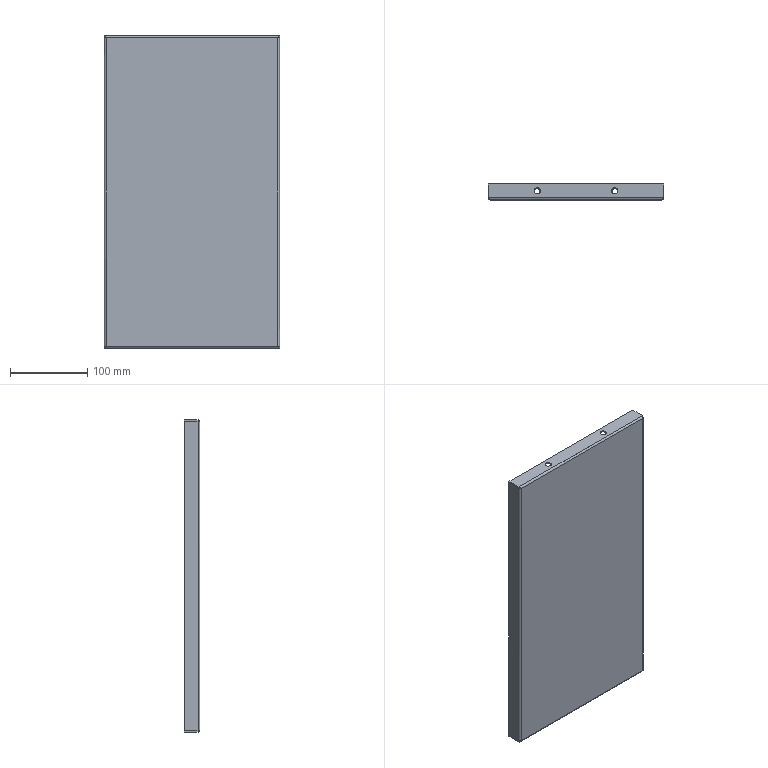Part | 1 solid | 46 faces | box 226 x 20 x 403 mm | volume 169868 mm3 | plane 22 | cylinder 16 | spline 8 | commonest cylinder face diameters 1.473 x4 4.473 x4 6.8 x4 8 x4